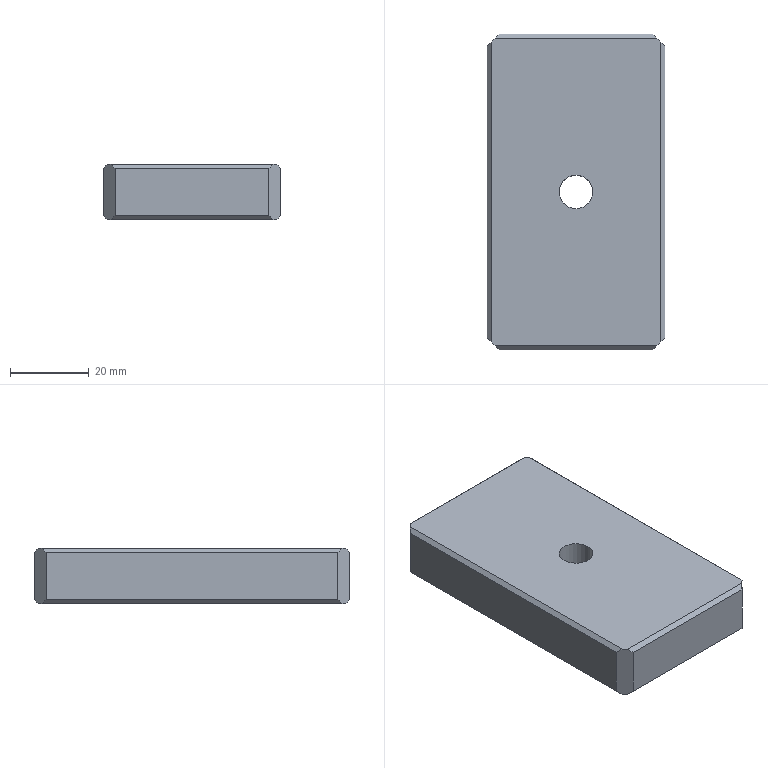Part | NX | 1 solid | 19 faces | box 45 x 80 x 14 mm | volume 49125 mm3 | plane 18 | cylinder 1 | commonest cylinder face diameters 8.5 x1
STEP:
#1=CARTESIAN_POINT('',(-17.,50.,13.));
#2=VERTEX_POINT('',#1);
#3=CARTESIAN_POINT('',(22.,50.,13.));
#4=VERTEX_POINT('',#3);
#5=CARTESIAN_POINT('',(25.,50.,13.));
#6=DIRECTION('',(1.,0.,0.));
#7=VECTOR('',#6,1000.);
#8=LINE('',#5,#7);
#9=EDGE_CURVE('',#2,#4,#8,.T.);
#10=ORIENTED_EDGE('',*,*,#9,.T.);
#11=CARTESIAN_POINT('',(22.,50.,1.));
#12=VERTEX_POINT('',#11);
#13=CARTESIAN_POINT('',(22.,50.,14.));
#14=DIRECTION('',(0.,0.,-1.));
#15=VECTOR('',#14,1000.);
#16=LINE('',#13,#15);
#17=EDGE_CURVE('',#4,#12,#16,.T.);
#18=ORIENTED_EDGE('',*,*,#17,.T.);
#19=CARTESIAN_POINT('',(-17.,50.,1.));
#20=VERTEX_POINT('',#19);
#21=CARTESIAN_POINT('',(25.,50.,1.));
#22=DIRECTION('',(-1.,0.,0.));
#23=VECTOR('',#22,1000.);
#24=LINE('',#21,#23);
#25=EDGE_CURVE('',#12,#20,#24,.T.);
#26=ORIENTED_EDGE('',*,*,#25,.T.);
#27=CARTESIAN_POINT('',(-17.,50.,14.));
#28=DIRECTION('',(0.,0.,1.));
#29=VECTOR('',#28,1000.);
#30=LINE('',#27,#29);
#31=EDGE_CURVE('',#20,#2,#30,.T.);
#32=ORIENTED_EDGE('',*,*,#31,.T.);
#33=EDGE_LOOP('',(#10,#18,#26,#32));
#34=FACE_BOUND('',#33,.T.);
#35=CARTESIAN_POINT('',(25.,50.,14.));
#36=DIRECTION('',(0.,-1.,0.));
#37=DIRECTION('',(0.,0.,-1.));
#38=AXIS2_PLACEMENT_3D('',#35,#36,#37);
#39=PLANE('',#38);
#40=ADVANCED_FACE('',(#34),#39,.F.);
#41=CARTESIAN_POINT('',(-20.,-27.,13.));
#42=VERTEX_POINT('',#41);
#43=CARTESIAN_POINT('',(-20.,47.,13.));
#44=VERTEX_POINT('',#43);
#45=CARTESIAN_POINT('',(-20.,50.,13.));
#46=DIRECTION('',(0.,1.,0.));
#47=VECTOR('',#46,1000.);
#48=LINE('',#45,#47);
#49=EDGE_CURVE('',#42,#44,#48,.T.);
#50=ORIENTED_EDGE('',*,*,#49,.T.);
#51=CARTESIAN_POINT('',(-20.,47.,1.));
#52=VERTEX_POINT('',#51);
#53=CARTESIAN_POINT('',(-20.,47.,14.));
#54=DIRECTION('',(0.,0.,-1.));
#55=VECTOR('',#54,1000.);
#56=LINE('',#53,#55);
#57=EDGE_CURVE('',#44,#52,#56,.T.);
#58=ORIENTED_EDGE('',*,*,#57,.T.);
#59=CARTESIAN_POINT('',(-20.,-27.,1.));
#60=VERTEX_POINT('',#59);
#61=CARTESIAN_POINT('',(-20.,50.,1.));
#62=DIRECTION('',(0.,-1.,0.));
#63=VECTOR('',#62,1000.);
#64=LINE('',#61,#63);
#65=EDGE_CURVE('',#52,#60,#64,.T.);
#66=ORIENTED_EDGE('',*,*,#65,.T.);
#67=CARTESIAN_POINT('',(-20.,-27.,14.));
#68=DIRECTION('',(0.,0.,1.));
#69=VECTOR('',#68,1000.);
#70=LINE('',#67,#69);
#71=EDGE_CURVE('',#60,#42,#70,.T.);
#72=ORIENTED_EDGE('',*,*,#71,.T.);
#73=EDGE_LOOP('',(#50,#58,#66,#72));
#74=FACE_BOUND('',#73,.T.);
#75=CARTESIAN_POINT('',(-20.,50.,14.));
#76=DIRECTION('',(1.,0.,0.));
#77=DIRECTION('',(0.,1.,0.));
#78=AXIS2_PLACEMENT_3D('',#75,#76,#77);
#79=PLANE('',#78);
#80=ADVANCED_FACE('',(#74),#79,.F.);
#81=CARTESIAN_POINT('',(22.,-30.,13.));
#82=VERTEX_POINT('',#81);
#83=CARTESIAN_POINT('',(-17.,-30.,13.));
#84=VERTEX_POINT('',#83);
#85=CARTESIAN_POINT('',(-20.,-30.,13.));
#86=DIRECTION('',(-1.,0.,0.));
#87=VECTOR('',#86,1000.);
#88=LINE('',#85,#87);
#89=EDGE_CURVE('',#82,#84,#88,.T.);
#90=ORIENTED_EDGE('',*,*,#89,.T.);
#91=CARTESIAN_POINT('',(-17.,-30.,1.));
#92=VERTEX_POINT('',#91);
#93=CARTESIAN_POINT('',(-17.,-30.,14.));
#94=DIRECTION('',(0.,0.,-1.));
#95=VECTOR('',#94,1000.);
#96=LINE('',#93,#95);
#97=EDGE_CURVE('',#84,#92,#96,.T.);
#98=ORIENTED_EDGE('',*,*,#97,.T.);
#99=CARTESIAN_POINT('',(22.,-30.,1.));
#100=VERTEX_POINT('',#99);
#101=CARTESIAN_POINT('',(-20.,-30.,1.));
#102=DIRECTION('',(1.,0.,0.));
#103=VECTOR('',#102,1000.);
#104=LINE('',#101,#103);
#105=EDGE_CURVE('',#92,#100,#104,.T.);
#106=ORIENTED_EDGE('',*,*,#105,.T.);
#107=CARTESIAN_POINT('',(22.,-30.,14.));
#108=DIRECTION('',(0.,0.,1.));
#109=VECTOR('',#108,1000.);
#110=LINE('',#107,#109);
#111=EDGE_CURVE('',#100,#82,#110,.T.);
#112=ORIENTED_EDGE('',*,*,#111,.T.);
#113=EDGE_LOOP('',(#90,#98,#106,#112));
#114=FACE_BOUND('',#113,.T.);
#115=CARTESIAN_POINT('',(-20.,-30.,14.));
#116=DIRECTION('',(0.,1.,0.));
#117=DIRECTION('',(-1.,0.,0.));
#118=AXIS2_PLACEMENT_3D('',#115,#116,#117);
#119=PLANE('',#118);
#120=ADVANCED_FACE('',(#114),#119,.F.);
#121=CARTESIAN_POINT('',(25.,-27.,1.));
#122=VERTEX_POINT('',#121);
#123=CARTESIAN_POINT('',(25.,47.,1.));
#124=VERTEX_POINT('',#123);
#125=CARTESIAN_POINT('',(25.,-30.,1.));
#126=DIRECTION('',(0.,1.,0.));
#127=VECTOR('',#126,1000.);
#128=LINE('',#125,#127);
#129=EDGE_CURVE('',#122,#124,#128,.T.);
#130=ORIENTED_EDGE('',*,*,#129,.T.);
#131=CARTESIAN_POINT('',(25.,47.,13.));
#132=VERTEX_POINT('',#131);
#133=CARTESIAN_POINT('',(25.,47.,14.));
#134=DIRECTION('',(0.,0.,1.));
#135=VECTOR('',#134,1000.);
#136=LINE('',#133,#135);
#137=EDGE_CURVE('',#124,#132,#136,.T.);
#138=ORIENTED_EDGE('',*,*,#137,.T.);
#139=CARTESIAN_POINT('',(25.,-27.,13.));
#140=VERTEX_POINT('',#139);
#141=CARTESIAN_POINT('',(25.,-30.,13.));
#142=DIRECTION('',(0.,-1.,0.));
#143=VECTOR('',#142,1000.);
#144=LINE('',#141,#143);
#145=EDGE_CURVE('',#132,#140,#144,.T.);
#146=ORIENTED_EDGE('',*,*,#145,.T.);
#147=CARTESIAN_POINT('',(25.,-27.,14.));
#148=DIRECTION('',(0.,0.,-1.));
#149=VECTOR('',#148,1000.);
#150=LINE('',#147,#149);
#151=EDGE_CURVE('',#140,#122,#150,.T.);
#152=ORIENTED_EDGE('',*,*,#151,.T.);
#153=EDGE_LOOP('',(#130,#138,#146,#152));
#154=FACE_BOUND('',#153,.T.);
#155=CARTESIAN_POINT('',(25.,-30.,14.));
#156=DIRECTION('',(-1.,0.,0.));
#157=DIRECTION('',(0.,-1.,0.));
#158=AXIS2_PLACEMENT_3D('',#155,#156,#157);
#159=PLANE('',#158);
#160=ADVANCED_FACE('',(#154),#159,.F.);
#161=CARTESIAN_POINT('',(6.75,10.,14.));
#162=VERTEX_POINT('',#161);
#163=CARTESIAN_POINT('',(2.5,10.,14.));
#164=DIRECTION('',(0.,0.,1.));
#165=DIRECTION('',(1.,0.,0.));
#166=AXIS2_PLACEMENT_3D('',#163,#164,#165);
#167=CIRCLE('',#166,4.25);
#168=EDGE_CURVE('',#162,#162,#167,.T.);
#169=ORIENTED_EDGE('',*,*,#168,.F.);
#170=EDGE_LOOP('',(#169));
#171=FACE_BOUND('',#170,.T.);
#172=CARTESIAN_POINT('',(24.,-28.,14.));
#173=VERTEX_POINT('',#172);
#174=CARTESIAN_POINT('',(24.,48.,14.));
#175=VERTEX_POINT('',#174);
#176=CARTESIAN_POINT('',(24.,50.,14.));
#177=DIRECTION('',(0.,1.,0.));
#178=VECTOR('',#177,1000.);
#179=LINE('',#176,#178);
#180=EDGE_CURVE('',#173,#175,#179,.T.);
#181=ORIENTED_EDGE('',*,*,#180,.T.);
#182=CARTESIAN_POINT('',(23.,49.,14.));
#183=VERTEX_POINT('',#182);
#184=CARTESIAN_POINT('',(36.,36.,14.));
#185=DIRECTION('',(0.7071,-0.7071,0.));
#186=VECTOR('',#185,1000.);
#187=LINE('',#184,#186);
#188=EDGE_CURVE('',#175,#183,#187,.F.);
#189=ORIENTED_EDGE('',*,*,#188,.T.);
#190=CARTESIAN_POINT('',(-18.,49.,14.));
#191=VERTEX_POINT('',#190);
#192=CARTESIAN_POINT('',(-20.,49.,14.));
#193=DIRECTION('',(-1.,0.,0.));
#194=VECTOR('',#193,1000.);
#195=LINE('',#192,#194);
#196=EDGE_CURVE('',#183,#191,#195,.T.);
#197=ORIENTED_EDGE('',*,*,#196,.T.);
#198=CARTESIAN_POINT('',(-19.,48.,14.));
#199=VERTEX_POINT('',#198);
#200=CARTESIAN_POINT('',(-33.5,33.5,14.));
#201=DIRECTION('',(0.7071,0.7071,0.));
#202=VECTOR('',#201,1000.);
#203=LINE('',#200,#202);
#204=EDGE_CURVE('',#191,#199,#203,.F.);
#205=ORIENTED_EDGE('',*,*,#204,.T.);
#206=CARTESIAN_POINT('',(-19.,-28.,14.));
#207=VERTEX_POINT('',#206);
#208=CARTESIAN_POINT('',(-19.,-30.,14.));
#209=DIRECTION('',(0.,-1.,0.));
#210=VECTOR('',#209,1000.);
#211=LINE('',#208,#210);
#212=EDGE_CURVE('',#199,#207,#211,.T.);
#213=ORIENTED_EDGE('',*,*,#212,.T.);
#214=CARTESIAN_POINT('',(-18.,-29.,14.));
#215=VERTEX_POINT('',#214);
#216=CARTESIAN_POINT('',(-23.5,-23.5,14.));
#217=DIRECTION('',(-0.7071,0.7071,0.));
#218=VECTOR('',#217,1000.);
#219=LINE('',#216,#218);
#220=EDGE_CURVE('',#207,#215,#219,.F.);
#221=ORIENTED_EDGE('',*,*,#220,.T.);
#222=CARTESIAN_POINT('',(23.,-29.,14.));
#223=VERTEX_POINT('',#222);
#224=CARTESIAN_POINT('',(25.,-29.,14.));
#225=DIRECTION('',(1.,0.,0.));
#226=VECTOR('',#225,1000.);
#227=LINE('',#224,#226);
#228=EDGE_CURVE('',#215,#223,#227,.T.);
#229=ORIENTED_EDGE('',*,*,#228,.T.);
#230=CARTESIAN_POINT('',(26.,-26.,14.));
#231=DIRECTION('',(-0.7071,-0.7071,0.));
#232=VECTOR('',#231,1000.);
#233=LINE('',#230,#232);
#234=EDGE_CURVE('',#223,#173,#233,.F.);
#235=ORIENTED_EDGE('',*,*,#234,.T.);
#236=EDGE_LOOP('',(#181,#189,#197,#205,#213,#221,#229,#235));
#237=FACE_BOUND('',#236,.T.);
#238=CARTESIAN_POINT('',(0.,0.,14.));
#239=DIRECTION('',(0.,0.,1.));
#240=DIRECTION('',(1.,0.,0.));
#241=AXIS2_PLACEMENT_3D('',#238,#239,#240);
#242=PLANE('',#241);
#243=ADVANCED_FACE('',(#171,#237),#242,.T.);
#244=CARTESIAN_POINT('',(6.75,10.,0.));
#245=VERTEX_POINT('',#244);
#246=CARTESIAN_POINT('',(2.5,10.,0.));
#247=DIRECTION('',(0.,0.,1.));
#248=DIRECTION('',(1.,0.,0.));
#249=AXIS2_PLACEMENT_3D('',#246,#247,#248);
#250=CIRCLE('',#249,4.25);
#251=EDGE_CURVE('',#245,#245,#250,.T.);
#252=ORIENTED_EDGE('',*,*,#251,.T.);
#253=EDGE_LOOP('',(#252));
#254=FACE_BOUND('',#253,.T.);
#255=CARTESIAN_POINT('',(-18.,49.,0.));
#256=VERTEX_POINT('',#255);
#257=CARTESIAN_POINT('',(23.,49.,0.));
#258=VERTEX_POINT('',#257);
#259=CARTESIAN_POINT('',(0.,49.,0.));
#260=DIRECTION('',(1.,0.,0.));
#261=VECTOR('',#260,1000.);
#262=LINE('',#259,#261);
#263=EDGE_CURVE('',#256,#258,#262,.T.);
#264=ORIENTED_EDGE('',*,*,#263,.T.);
#265=CARTESIAN_POINT('',(24.,48.,0.));
#266=VERTEX_POINT('',#265);
#267=CARTESIAN_POINT('',(22.,50.,0.));
#268=DIRECTION('',(-0.7071,0.7071,0.));
#269=VECTOR('',#268,1000.);
#270=LINE('',#267,#269);
#271=EDGE_CURVE('',#258,#266,#270,.F.);
#272=ORIENTED_EDGE('',*,*,#271,.T.);
#273=CARTESIAN_POINT('',(24.,-28.,0.));
#274=VERTEX_POINT('',#273);
#275=CARTESIAN_POINT('',(24.,0.,0.));
#276=DIRECTION('',(0.,-1.,0.));
#277=VECTOR('',#276,1000.);
#278=LINE('',#275,#277);
#279=EDGE_CURVE('',#266,#274,#278,.T.);
#280=ORIENTED_EDGE('',*,*,#279,.T.);
#281=CARTESIAN_POINT('',(23.,-29.,0.));
#282=VERTEX_POINT('',#281);
#283=CARTESIAN_POINT('',(25.,-27.,0.));
#284=DIRECTION('',(0.7071,0.7071,0.));
#285=VECTOR('',#284,1000.);
#286=LINE('',#283,#285);
#287=EDGE_CURVE('',#274,#282,#286,.F.);
#288=ORIENTED_EDGE('',*,*,#287,.T.);
#289=CARTESIAN_POINT('',(-18.,-29.,0.));
#290=VERTEX_POINT('',#289);
#291=CARTESIAN_POINT('',(0.,-29.,0.));
#292=DIRECTION('',(-1.,0.,0.));
#293=VECTOR('',#292,1000.);
#294=LINE('',#291,#293);
#295=EDGE_CURVE('',#282,#290,#294,.T.);
#296=ORIENTED_EDGE('',*,*,#295,.T.);
#297=CARTESIAN_POINT('',(-19.,-28.,0.));
#298=VERTEX_POINT('',#297);
#299=CARTESIAN_POINT('',(-17.,-30.,0.));
#300=DIRECTION('',(0.7071,-0.7071,0.));
#301=VECTOR('',#300,1000.);
#302=LINE('',#299,#301);
#303=EDGE_CURVE('',#290,#298,#302,.F.);
#304=ORIENTED_EDGE('',*,*,#303,.T.);
#305=CARTESIAN_POINT('',(-19.,48.,0.));
#306=VERTEX_POINT('',#305);
#307=CARTESIAN_POINT('',(-19.,0.,0.));
#308=DIRECTION('',(0.,1.,0.));
#309=VECTOR('',#308,1000.);
#310=LINE('',#307,#309);
#311=EDGE_CURVE('',#298,#306,#310,.T.);
#312=ORIENTED_EDGE('',*,*,#311,.T.);
#313=CARTESIAN_POINT('',(-20.,47.,0.));
#314=DIRECTION('',(-0.7071,-0.7071,0.));
#315=VECTOR('',#314,1000.);
#316=LINE('',#313,#315);
#317=EDGE_CURVE('',#306,#256,#316,.F.);
#318=ORIENTED_EDGE('',*,*,#317,.T.);
#319=EDGE_LOOP('',(#264,#272,#280,#288,#296,#304,#312,#318));
#320=FACE_BOUND('',#319,.T.);
#321=CARTESIAN_POINT('',(0.,0.,0.));
#322=DIRECTION('',(0.,0.,1.));
#323=DIRECTION('',(1.,0.,0.));
#324=AXIS2_PLACEMENT_3D('',#321,#322,#323);
#325=PLANE('',#324);
#326=ADVANCED_FACE('',(#254,#320),#325,.F.);
#327=ORIENTED_EDGE('',*,*,#105,.F.);
#328=CARTESIAN_POINT('',(-18.,-29.,0.));
#329=DIRECTION('',(-0.5774,0.5774,-0.5774));
#330=VECTOR('',#329,1000.);
#331=LINE('',#328,#330);
#332=EDGE_CURVE('',#92,#290,#331,.T.);
#333=ORIENTED_EDGE('',*,*,#332,.T.);
#334=ORIENTED_EDGE('',*,*,#295,.F.);
#335=CARTESIAN_POINT('',(8.,-44.,15.));
#336=DIRECTION('',(-0.5774,-0.5774,0.5774));
#337=VECTOR('',#336,1000.);
#338=LINE('',#335,#337);
#339=EDGE_CURVE('',#282,#100,#338,.T.);
#340=ORIENTED_EDGE('',*,*,#339,.T.);
#341=EDGE_LOOP('',(#327,#333,#334,#340));
#342=FACE_BOUND('',#341,.T.);
#343=CARTESIAN_POINT('',(-20.,-30.,1.));
#344=DIRECTION('',(0.,0.7071,0.7071));
#345=DIRECTION('',(1.,0.,0.));
#346=AXIS2_PLACEMENT_3D('',#343,#344,#345);
#347=PLANE('',#346);
#348=ADVANCED_FACE('',(#342),#347,.F.);
#349=ORIENTED_EDGE('',*,*,#279,.F.);
#350=CARTESIAN_POINT('',(50.667,21.333,26.667));
#351=DIRECTION('',(0.5774,-0.5774,0.5774));
#352=VECTOR('',#351,1000.);
#353=LINE('',#350,#352);
#354=EDGE_CURVE('',#266,#124,#353,.T.);
#355=ORIENTED_EDGE('',*,*,#354,.T.);
#356=ORIENTED_EDGE('',*,*,#129,.F.);
#357=CARTESIAN_POINT('',(24.,-28.,0.));
#358=DIRECTION('',(-0.5774,-0.5774,-0.5774));
#359=VECTOR('',#358,1000.);
#360=LINE('',#357,#359);
#361=EDGE_CURVE('',#122,#274,#360,.T.);
#362=ORIENTED_EDGE('',*,*,#361,.T.);
#363=EDGE_LOOP('',(#349,#355,#356,#362));
#364=FACE_BOUND('',#363,.T.);
#365=CARTESIAN_POINT('',(25.,-30.,1.));
#366=DIRECTION('',(-0.7071,0.,0.7071));
#367=DIRECTION('',(0.,1.,0.));
#368=AXIS2_PLACEMENT_3D('',#365,#366,#367);
#369=PLANE('',#368);
#370=ADVANCED_FACE('',(#364),#369,.F.);
#371=ORIENTED_EDGE('',*,*,#65,.F.);
#372=CARTESIAN_POINT('',(-19.,48.,0.));
#373=DIRECTION('',(0.5774,0.5774,-0.5774));
#374=VECTOR('',#373,1000.);
#375=LINE('',#372,#374);
#376=EDGE_CURVE('',#52,#306,#375,.T.);
#377=ORIENTED_EDGE('',*,*,#376,.T.);
#378=ORIENTED_EDGE('',*,*,#311,.F.);
#379=CARTESIAN_POINT('',(-45.667,-1.333,26.667));
#380=DIRECTION('',(-0.5774,0.5774,0.5774));
#381=VECTOR('',#380,1000.);
#382=LINE('',#379,#381);
#383=EDGE_CURVE('',#298,#60,#382,.T.);
#384=ORIENTED_EDGE('',*,*,#383,.T.);
#385=EDGE_LOOP('',(#371,#377,#378,#384));
#386=FACE_BOUND('',#385,.T.);
#387=CARTESIAN_POINT('',(-20.,50.,1.));
#388=DIRECTION('',(0.7071,0.,0.7071));
#389=DIRECTION('',(0.,-1.,0.));
#390=AXIS2_PLACEMENT_3D('',#387,#388,#389);
#391=PLANE('',#390);
#392=ADVANCED_FACE('',(#386),#391,.F.);
#393=ORIENTED_EDGE('',*,*,#25,.F.);
#394=CARTESIAN_POINT('',(23.,49.,0.));
#395=DIRECTION('',(0.5774,-0.5774,-0.5774));
#396=VECTOR('',#395,1000.);
#397=LINE('',#394,#396);
#398=EDGE_CURVE('',#12,#258,#397,.T.);
#399=ORIENTED_EDGE('',*,*,#398,.T.);
#400=ORIENTED_EDGE('',*,*,#263,.F.);
#401=CARTESIAN_POINT('',(-3.,64.,15.));
#402=DIRECTION('',(0.5774,0.5774,0.5774));
#403=VECTOR('',#402,1000.);
#404=LINE('',#401,#403);
#405=EDGE_CURVE('',#256,#20,#404,.T.);
#406=ORIENTED_EDGE('',*,*,#405,.T.);
#407=EDGE_LOOP('',(#393,#399,#400,#406));
#408=FACE_BOUND('',#407,.T.);
#409=CARTESIAN_POINT('',(25.,50.,1.));
#410=DIRECTION('',(0.,-0.7071,0.7071));
#411=DIRECTION('',(-1.,0.,0.));
#412=AXIS2_PLACEMENT_3D('',#409,#410,#411);
#413=PLANE('',#412);
#414=ADVANCED_FACE('',(#408),#413,.F.);
#415=ORIENTED_EDGE('',*,*,#228,.F.);
#416=CARTESIAN_POINT('',(-12.,-35.,8.));
#417=DIRECTION('',(-0.5774,0.5774,0.5774));
#418=VECTOR('',#417,1000.);
#419=LINE('',#416,#418);
#420=EDGE_CURVE('',#215,#84,#419,.F.);
#421=ORIENTED_EDGE('',*,*,#420,.T.);
#422=ORIENTED_EDGE('',*,*,#89,.F.);
#423=CARTESIAN_POINT('',(15.333,-36.667,6.333));
#424=DIRECTION('',(-0.5774,-0.5774,-0.5774));
#425=VECTOR('',#424,1000.);
#426=LINE('',#423,#425);
#427=EDGE_CURVE('',#82,#223,#426,.F.);
#428=ORIENTED_EDGE('',*,*,#427,.T.);
#429=EDGE_LOOP('',(#415,#421,#422,#428));
#430=FACE_BOUND('',#429,.T.);
#431=CARTESIAN_POINT('',(0.,-29.,14.));
#432=DIRECTION('',(0.,-0.7071,0.7071));
#433=DIRECTION('',(-1.,0.,0.));
#434=AXIS2_PLACEMENT_3D('',#431,#432,#433);
#435=PLANE('',#434);
#436=ADVANCED_FACE('',(#430),#435,.T.);
#437=ORIENTED_EDGE('',*,*,#145,.F.);
#438=CARTESIAN_POINT('',(40.,32.,-2.));
#439=DIRECTION('',(0.5774,-0.5774,-0.5774));
#440=VECTOR('',#439,1000.);
#441=LINE('',#438,#440);
#442=EDGE_CURVE('',#132,#175,#441,.F.);
#443=ORIENTED_EDGE('',*,*,#442,.T.);
#444=ORIENTED_EDGE('',*,*,#180,.F.);
#445=CARTESIAN_POINT('',(33.333,-18.667,4.667));
#446=DIRECTION('',(-0.5774,-0.5774,0.5774));
#447=VECTOR('',#446,1000.);
#448=LINE('',#445,#447);
#449=EDGE_CURVE('',#173,#140,#448,.F.);
#450=ORIENTED_EDGE('',*,*,#449,.T.);
#451=EDGE_LOOP('',(#437,#443,#444,#450));
#452=FACE_BOUND('',#451,.T.);
#453=CARTESIAN_POINT('',(24.,0.,14.));
#454=DIRECTION('',(0.7071,0.,0.7071));
#455=DIRECTION('',(0.,-1.,0.));
#456=AXIS2_PLACEMENT_3D('',#453,#454,#455);
#457=PLANE('',#456);
#458=ADVANCED_FACE('',(#452),#457,.T.);
#459=ORIENTED_EDGE('',*,*,#212,.F.);
#460=CARTESIAN_POINT('',(-35.,32.,-2.));
#461=DIRECTION('',(0.5774,0.5774,0.5774));
#462=VECTOR('',#461,1000.);
#463=LINE('',#460,#462);
#464=EDGE_CURVE('',#199,#44,#463,.F.);
#465=ORIENTED_EDGE('',*,*,#464,.T.);
#466=ORIENTED_EDGE('',*,*,#49,.F.);
#467=CARTESIAN_POINT('',(-28.333,-18.667,4.667));
#468=DIRECTION('',(-0.5774,0.5774,-0.5774));
#469=VECTOR('',#468,1000.);
#470=LINE('',#467,#469);
#471=EDGE_CURVE('',#42,#207,#470,.F.);
#472=ORIENTED_EDGE('',*,*,#471,.T.);
#473=EDGE_LOOP('',(#459,#465,#466,#472));
#474=FACE_BOUND('',#473,.T.);
#475=CARTESIAN_POINT('',(-19.,0.,14.));
#476=DIRECTION('',(-0.7071,0.,0.7071));
#477=DIRECTION('',(0.,1.,0.));
#478=AXIS2_PLACEMENT_3D('',#475,#476,#477);
#479=PLANE('',#478);
#480=ADVANCED_FACE('',(#474),#479,.T.);
#481=ORIENTED_EDGE('',*,*,#196,.F.);
#482=CARTESIAN_POINT('',(15.333,56.667,6.333));
#483=DIRECTION('',(0.5774,-0.5774,0.5774));
#484=VECTOR('',#483,1000.);
#485=LINE('',#482,#484);
#486=EDGE_CURVE('',#183,#4,#485,.F.);
#487=ORIENTED_EDGE('',*,*,#486,.T.);
#488=ORIENTED_EDGE('',*,*,#9,.F.);
#489=CARTESIAN_POINT('',(-12.,55.,8.));
#490=DIRECTION('',(0.5774,0.5774,-0.5774));
#491=VECTOR('',#490,1000.);
#492=LINE('',#489,#491);
#493=EDGE_CURVE('',#2,#191,#492,.F.);
#494=ORIENTED_EDGE('',*,*,#493,.T.);
#495=EDGE_LOOP('',(#481,#487,#488,#494));
#496=FACE_BOUND('',#495,.T.);
#497=CARTESIAN_POINT('',(0.,49.,14.));
#498=DIRECTION('',(0.,0.7071,0.7071));
#499=DIRECTION('',(1.,0.,0.));
#500=AXIS2_PLACEMENT_3D('',#497,#498,#499);
#501=PLANE('',#500);
#502=ADVANCED_FACE('',(#496),#501,.T.);
#503=ORIENTED_EDGE('',*,*,#442,.F.);
#504=ORIENTED_EDGE('',*,*,#137,.F.);
#505=ORIENTED_EDGE('',*,*,#354,.F.);
#506=ORIENTED_EDGE('',*,*,#271,.F.);
#507=ORIENTED_EDGE('',*,*,#398,.F.);
#508=ORIENTED_EDGE('',*,*,#17,.F.);
#509=ORIENTED_EDGE('',*,*,#486,.F.);
#510=ORIENTED_EDGE('',*,*,#188,.F.);
#511=EDGE_LOOP('',(#503,#504,#505,#506,#507,#508,#509,#510));
#512=FACE_BOUND('',#511,.T.);
#513=CARTESIAN_POINT('',(22.,50.,14.));
#514=DIRECTION('',(-0.7071,-0.7071,0.));
#515=DIRECTION('',(0.,0.,-1.));
#516=AXIS2_PLACEMENT_3D('',#513,#514,#515);
#517=PLANE('',#516);
#518=ADVANCED_FACE('',(#512),#517,.F.);
#519=ORIENTED_EDGE('',*,*,#493,.F.);
#520=ORIENTED_EDGE('',*,*,#31,.F.);
#521=ORIENTED_EDGE('',*,*,#405,.F.);
#522=ORIENTED_EDGE('',*,*,#317,.F.);
#523=ORIENTED_EDGE('',*,*,#376,.F.);
#524=ORIENTED_EDGE('',*,*,#57,.F.);
#525=ORIENTED_EDGE('',*,*,#464,.F.);
#526=ORIENTED_EDGE('',*,*,#204,.F.);
#527=EDGE_LOOP('',(#519,#520,#521,#522,#523,#524,#525,#526));
#528=FACE_BOUND('',#527,.T.);
#529=CARTESIAN_POINT('',(-20.,47.,14.));
#530=DIRECTION('',(0.7071,-0.7071,0.));
#531=DIRECTION('',(0.,0.,-1.));
#532=AXIS2_PLACEMENT_3D('',#529,#530,#531);
#533=PLANE('',#532);
#534=ADVANCED_FACE('',(#528),#533,.F.);
#535=ORIENTED_EDGE('',*,*,#471,.F.);
#536=ORIENTED_EDGE('',*,*,#71,.F.);
#537=ORIENTED_EDGE('',*,*,#383,.F.);
#538=ORIENTED_EDGE('',*,*,#303,.F.);
#539=ORIENTED_EDGE('',*,*,#332,.F.);
#540=ORIENTED_EDGE('',*,*,#97,.F.);
#541=ORIENTED_EDGE('',*,*,#420,.F.);
#542=ORIENTED_EDGE('',*,*,#220,.F.);
#543=EDGE_LOOP('',(#535,#536,#537,#538,#539,#540,#541,#542));
#544=FACE_BOUND('',#543,.T.);
#545=CARTESIAN_POINT('',(-17.,-30.,14.));
#546=DIRECTION('',(0.7071,0.7071,0.));
#547=DIRECTION('',(0.,0.,-1.));
#548=AXIS2_PLACEMENT_3D('',#545,#546,#547);
#549=PLANE('',#548);
#550=ADVANCED_FACE('',(#544),#549,.F.);
#551=ORIENTED_EDGE('',*,*,#427,.F.);
#552=ORIENTED_EDGE('',*,*,#111,.F.);
#553=ORIENTED_EDGE('',*,*,#339,.F.);
#554=ORIENTED_EDGE('',*,*,#287,.F.);
#555=ORIENTED_EDGE('',*,*,#361,.F.);
#556=ORIENTED_EDGE('',*,*,#151,.F.);
#557=ORIENTED_EDGE('',*,*,#449,.F.);
#558=ORIENTED_EDGE('',*,*,#234,.F.);
#559=EDGE_LOOP('',(#551,#552,#553,#554,#555,#556,#557,#558));
#560=FACE_BOUND('',#559,.T.);
#561=CARTESIAN_POINT('',(25.,-27.,14.));
#562=DIRECTION('',(-0.7071,0.7071,0.));
#563=DIRECTION('',(0.,0.,-1.));
#564=AXIS2_PLACEMENT_3D('',#561,#562,#563);
#565=PLANE('',#564);
#566=ADVANCED_FACE('',(#560),#565,.F.);
#567=ORIENTED_EDGE('',*,*,#251,.F.);
#568=EDGE_LOOP('',(#567));
#569=FACE_BOUND('',#568,.T.);
#570=ORIENTED_EDGE('',*,*,#168,.T.);
#571=EDGE_LOOP('',(#570));
#572=FACE_BOUND('',#571,.T.);
#573=CARTESIAN_POINT('',(2.5,10.,14.));
#574=DIRECTION('',(0.,0.,1.));
#575=DIRECTION('',(1.,0.,0.));
#576=AXIS2_PLACEMENT_3D('',#573,#574,#575);
#577=CYLINDRICAL_SURFACE('',#576,4.25);
#578=ADVANCED_FACE('',(#569,#572),#577,.F.);
#579=CLOSED_SHELL('',(#40,#80,#120,#160,#243,#326,#348,#370,#392,#414,#436,#458,#480,#502,#518,#534,#550,#566,#578));
#580=MANIFOLD_SOLID_BREP('',#579);
#581=(LENGTH_UNIT()NAMED_UNIT(*)SI_UNIT(.MILLI.,.METRE.));
#582=UNCERTAINTY_MEASURE_WITH_UNIT(LENGTH_MEASURE(0.00001),#581,'','');
#583=(NAMED_UNIT(*)PLANE_ANGLE_UNIT()SI_UNIT($,.RADIAN.));
#584=(NAMED_UNIT(*)SI_UNIT($,.STERADIAN.)SOLID_ANGLE_UNIT());
#585=(GEOMETRIC_REPRESENTATION_CONTEXT(3)GLOBAL_UNCERTAINTY_ASSIGNED_CONTEXT((#582))GLOBAL_UNIT_ASSIGNED_CONTEXT((#581,#583,#584))REPRESENTATION_CONTEXT('',''));
#586=ADVANCED_BREP_SHAPE_REPRESENTATION('',(#580),#585);